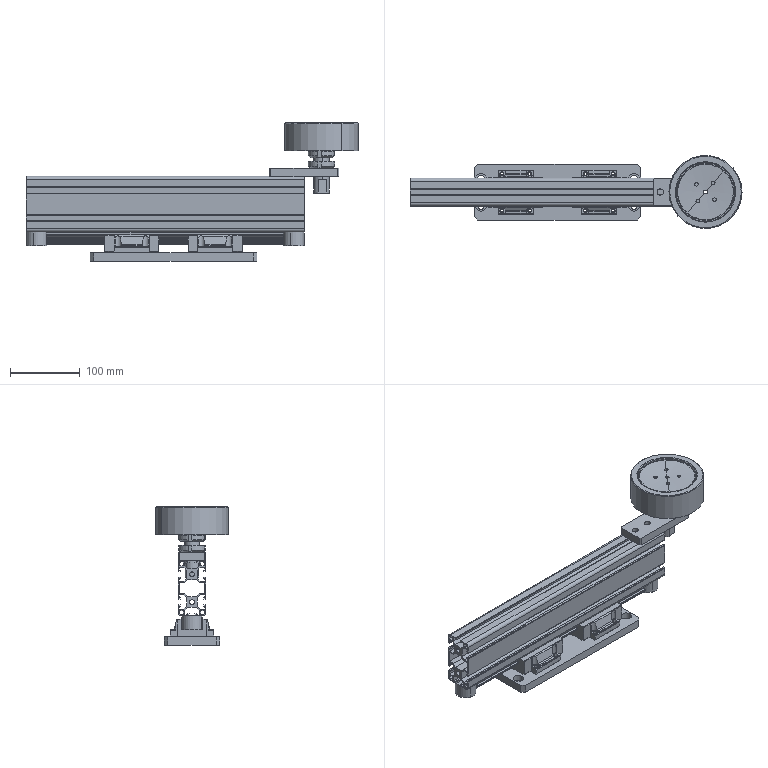Part | SolidWorks | 12 solids | 1254 faces | box 477.5 x 105 x 199 mm | volume 1081660 mm3 | plane 831 | cylinder 229 | spline 145 | cone 47 | torus 2 | commonest cylinder face diameters 1 x36 6 x28 2 x22 9 x17 4.2 x16 4.06 x12